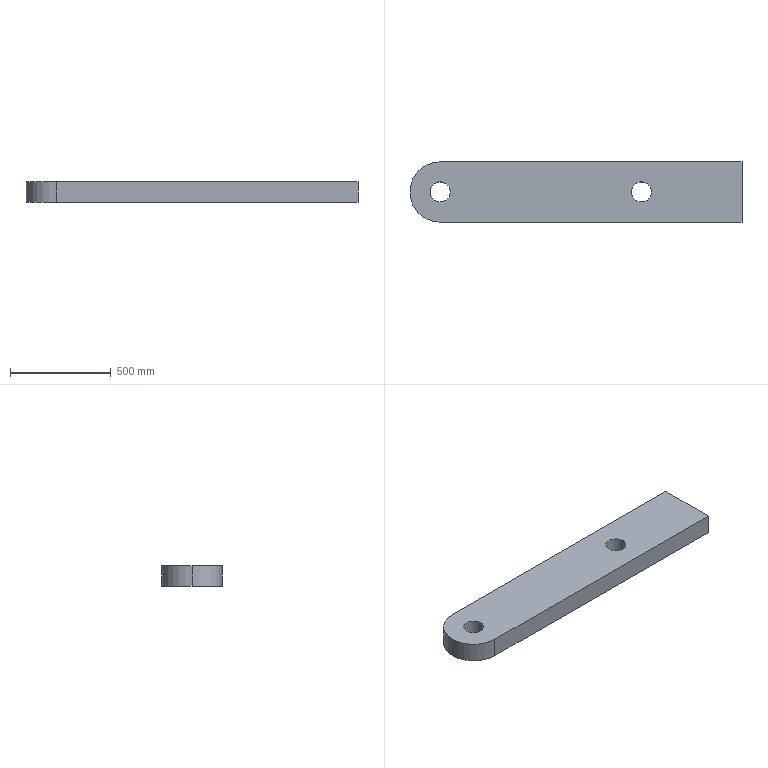Part | SolidWorks | features Extrusion 1 | 1 solid | 11 faces | box 1650 x 300 x 100 mm | volume 46963495 mm3 | cylinder 6 | plane 5 | commonest cylinder face diameters 100 x4 300 x2
STEP:
#1=CARTESIAN_POINT('',(-50.,0.,100.));
#2=VERTEX_POINT('',#1);
#3=CARTESIAN_POINT('',(50.,0.,100.));
#4=VERTEX_POINT('',#3);
#5=CARTESIAN_POINT('',(0.,0.,100.));
#6=DIRECTION('',(0.,0.,1.));
#7=DIRECTION('',(1.,0.,0.));
#8=AXIS2_PLACEMENT_3D('',#5,#6,#7);
#9=CIRCLE('',#8,50.);
#10=EDGE_CURVE('',#2,#4,#9,.T.);
#11=ORIENTED_EDGE('',*,*,#10,.T.);
#12=CARTESIAN_POINT('',(50.,0.,0.));
#13=VERTEX_POINT('',#12);
#14=CARTESIAN_POINT('',(50.,0.,100.));
#15=DIRECTION('',(0.,0.,-1.));
#16=VECTOR('',#15,1000.);
#17=LINE('',#14,#16);
#18=EDGE_CURVE('',#4,#13,#17,.T.);
#19=ORIENTED_EDGE('',*,*,#18,.T.);
#20=CARTESIAN_POINT('',(-50.,0.,0.));
#21=VERTEX_POINT('',#20);
#22=CARTESIAN_POINT('',(0.,0.,0.));
#23=DIRECTION('',(0.,0.,1.));
#24=DIRECTION('',(1.,0.,0.));
#25=AXIS2_PLACEMENT_3D('',#22,#23,#24);
#26=CIRCLE('',#25,50.);
#27=EDGE_CURVE('',#21,#13,#26,.T.);
#28=ORIENTED_EDGE('',*,*,#27,.F.);
#29=CARTESIAN_POINT('',(-50.,0.,100.));
#30=DIRECTION('',(0.,0.,-1.));
#31=VECTOR('',#30,1000.);
#32=LINE('',#29,#31);
#33=EDGE_CURVE('',#2,#21,#32,.T.);
#34=ORIENTED_EDGE('',*,*,#33,.F.);
#35=EDGE_LOOP('',(#11,#19,#28,#34));
#36=FACE_OUTER_BOUND('',#35,.T.);
#37=CARTESIAN_POINT('',(0.,0.,100.));
#38=DIRECTION('',(0.,0.,-1.));
#39=DIRECTION('',(-1.,0.,0.));
#40=AXIS2_PLACEMENT_3D('',#37,#38,#39);
#41=CYLINDRICAL_SURFACE('',#40,50.);
#42=ADVANCED_FACE('',(#36),#41,.F.);
#43=CARTESIAN_POINT('',(950.,0.,100.));
#44=VERTEX_POINT('',#43);
#45=CARTESIAN_POINT('',(1050.,0.,100.));
#46=VERTEX_POINT('',#45);
#47=CARTESIAN_POINT('',(1000.,0.,100.));
#48=DIRECTION('',(0.,0.,1.));
#49=DIRECTION('',(1.,0.,0.));
#50=AXIS2_PLACEMENT_3D('',#47,#48,#49);
#51=CIRCLE('',#50,50.);
#52=EDGE_CURVE('',#44,#46,#51,.T.);
#53=ORIENTED_EDGE('',*,*,#52,.T.);
#54=CARTESIAN_POINT('',(1050.,0.,0.));
#55=VERTEX_POINT('',#54);
#56=CARTESIAN_POINT('',(1050.,0.,100.));
#57=DIRECTION('',(0.,0.,-1.));
#58=VECTOR('',#57,1000.);
#59=LINE('',#56,#58);
#60=EDGE_CURVE('',#46,#55,#59,.T.);
#61=ORIENTED_EDGE('',*,*,#60,.T.);
#62=CARTESIAN_POINT('',(950.,0.,0.));
#63=VERTEX_POINT('',#62);
#64=CARTESIAN_POINT('',(1000.,0.,0.));
#65=DIRECTION('',(0.,0.,1.));
#66=DIRECTION('',(1.,0.,0.));
#67=AXIS2_PLACEMENT_3D('',#64,#65,#66);
#68=CIRCLE('',#67,50.);
#69=EDGE_CURVE('',#63,#55,#68,.T.);
#70=ORIENTED_EDGE('',*,*,#69,.F.);
#71=CARTESIAN_POINT('',(950.,0.,100.));
#72=DIRECTION('',(0.,0.,-1.));
#73=VECTOR('',#72,1000.);
#74=LINE('',#71,#73);
#75=EDGE_CURVE('',#44,#63,#74,.T.);
#76=ORIENTED_EDGE('',*,*,#75,.F.);
#77=EDGE_LOOP('',(#53,#61,#70,#76));
#78=FACE_OUTER_BOUND('',#77,.T.);
#79=CARTESIAN_POINT('',(1000.,0.,100.));
#80=DIRECTION('',(0.,0.,-1.));
#81=DIRECTION('',(-1.,0.,0.));
#82=AXIS2_PLACEMENT_3D('',#79,#80,#81);
#83=CYLINDRICAL_SURFACE('',#82,50.);
#84=ADVANCED_FACE('',(#78),#83,.F.);
#85=CARTESIAN_POINT('',(-150.,0.,100.));
#86=VERTEX_POINT('',#85);
#87=CARTESIAN_POINT('',(0.,-150.,100.));
#88=VERTEX_POINT('',#87);
#89=CARTESIAN_POINT('',(0.,0.,100.));
#90=DIRECTION('',(0.,0.,1.));
#91=DIRECTION('',(1.,0.,0.));
#92=AXIS2_PLACEMENT_3D('',#89,#90,#91);
#93=CIRCLE('',#92,150.);
#94=EDGE_CURVE('',#86,#88,#93,.T.);
#95=ORIENTED_EDGE('',*,*,#94,.F.);
#96=CARTESIAN_POINT('',(-150.,0.,0.));
#97=VERTEX_POINT('',#96);
#98=CARTESIAN_POINT('',(-150.,0.,100.));
#99=DIRECTION('',(0.,0.,-1.));
#100=VECTOR('',#99,1000.);
#101=LINE('',#98,#100);
#102=EDGE_CURVE('',#86,#97,#101,.T.);
#103=ORIENTED_EDGE('',*,*,#102,.T.);
#104=CARTESIAN_POINT('',(0.,-150.,0.));
#105=VERTEX_POINT('',#104);
#106=CARTESIAN_POINT('',(0.,0.,0.));
#107=DIRECTION('',(0.,0.,1.));
#108=DIRECTION('',(1.,0.,0.));
#109=AXIS2_PLACEMENT_3D('',#106,#107,#108);
#110=CIRCLE('',#109,150.);
#111=EDGE_CURVE('',#97,#105,#110,.T.);
#112=ORIENTED_EDGE('',*,*,#111,.T.);
#113=CARTESIAN_POINT('',(0.,-150.,100.));
#114=DIRECTION('',(0.,0.,-1.));
#115=VECTOR('',#114,1000.);
#116=LINE('',#113,#115);
#117=EDGE_CURVE('',#88,#105,#116,.T.);
#118=ORIENTED_EDGE('',*,*,#117,.F.);
#119=EDGE_LOOP('',(#95,#103,#112,#118));
#120=FACE_OUTER_BOUND('',#119,.T.);
#121=CARTESIAN_POINT('',(0.,0.,100.));
#122=DIRECTION('',(0.,0.,-1.));
#123=DIRECTION('',(-1.,0.,0.));
#124=AXIS2_PLACEMENT_3D('',#121,#122,#123);
#125=CYLINDRICAL_SURFACE('',#124,150.);
#126=ADVANCED_FACE('',(#120),#125,.T.);
#127=ORIENTED_EDGE('',*,*,#52,.F.);
#128=CARTESIAN_POINT('',(1000.,0.,100.));
#129=DIRECTION('',(0.,0.,1.));
#130=DIRECTION('',(1.,0.,0.));
#131=AXIS2_PLACEMENT_3D('',#128,#129,#130);
#132=CIRCLE('',#131,50.);
#133=EDGE_CURVE('',#46,#44,#132,.T.);
#134=ORIENTED_EDGE('',*,*,#133,.F.);
#135=EDGE_LOOP('',(#127,#134));
#136=FACE_BOUND('',#135,.T.);
#137=CARTESIAN_POINT('',(0.,150.,100.));
#138=VERTEX_POINT('',#137);
#139=CARTESIAN_POINT('',(0.,0.,100.));
#140=DIRECTION('',(0.,0.,1.));
#141=DIRECTION('',(1.,0.,0.));
#142=AXIS2_PLACEMENT_3D('',#139,#140,#141);
#143=CIRCLE('',#142,150.);
#144=EDGE_CURVE('',#138,#86,#143,.T.);
#145=ORIENTED_EDGE('',*,*,#144,.T.);
#146=ORIENTED_EDGE('',*,*,#94,.T.);
#147=CARTESIAN_POINT('',(1500.,-150.,100.));
#148=VERTEX_POINT('',#147);
#149=CARTESIAN_POINT('',(1500.,-150.,100.));
#150=DIRECTION('',(1.,0.,0.));
#151=VECTOR('',#150,1000.);
#152=LINE('',#149,#151);
#153=EDGE_CURVE('',#88,#148,#152,.T.);
#154=ORIENTED_EDGE('',*,*,#153,.T.);
#155=CARTESIAN_POINT('',(1500.,150.,100.));
#156=VERTEX_POINT('',#155);
#157=CARTESIAN_POINT('',(1500.,150.,100.));
#158=DIRECTION('',(0.,1.,0.));
#159=VECTOR('',#158,1000.);
#160=LINE('',#157,#159);
#161=EDGE_CURVE('',#148,#156,#160,.T.);
#162=ORIENTED_EDGE('',*,*,#161,.T.);
#163=CARTESIAN_POINT('',(0.,150.,100.));
#164=DIRECTION('',(-1.,0.,0.));
#165=VECTOR('',#164,1000.);
#166=LINE('',#163,#165);
#167=EDGE_CURVE('',#156,#138,#166,.T.);
#168=ORIENTED_EDGE('',*,*,#167,.T.);
#169=EDGE_LOOP('',(#145,#146,#154,#162,#168));
#170=FACE_OUTER_BOUND('',#169,.T.);
#171=ORIENTED_EDGE('',*,*,#10,.F.);
#172=CARTESIAN_POINT('',(0.,0.,100.));
#173=DIRECTION('',(0.,0.,1.));
#174=DIRECTION('',(1.,0.,0.));
#175=AXIS2_PLACEMENT_3D('',#172,#173,#174);
#176=CIRCLE('',#175,50.);
#177=EDGE_CURVE('',#4,#2,#176,.T.);
#178=ORIENTED_EDGE('',*,*,#177,.F.);
#179=EDGE_LOOP('',(#171,#178));
#180=FACE_BOUND('',#179,.T.);
#181=CARTESIAN_POINT('',(0.,0.,100.));
#182=DIRECTION('',(0.,0.,1.));
#183=DIRECTION('',(1.,0.,0.));
#184=AXIS2_PLACEMENT_3D('',#181,#182,#183);
#185=PLANE('',#184);
#186=ADVANCED_FACE('',(#136,#170,#180),#185,.T.);
#187=ORIENTED_EDGE('',*,*,#69,.T.);
#188=CARTESIAN_POINT('',(1000.,0.,0.));
#189=DIRECTION('',(0.,0.,1.));
#190=DIRECTION('',(1.,0.,0.));
#191=AXIS2_PLACEMENT_3D('',#188,#189,#190);
#192=CIRCLE('',#191,50.);
#193=EDGE_CURVE('',#55,#63,#192,.T.);
#194=ORIENTED_EDGE('',*,*,#193,.T.);
#195=EDGE_LOOP('',(#187,#194));
#196=FACE_BOUND('',#195,.T.);
#197=CARTESIAN_POINT('',(0.,150.,0.));
#198=VERTEX_POINT('',#197);
#199=CARTESIAN_POINT('',(0.,0.,0.));
#200=DIRECTION('',(0.,0.,1.));
#201=DIRECTION('',(1.,0.,0.));
#202=AXIS2_PLACEMENT_3D('',#199,#200,#201);
#203=CIRCLE('',#202,150.);
#204=EDGE_CURVE('',#198,#97,#203,.T.);
#205=ORIENTED_EDGE('',*,*,#204,.F.);
#206=CARTESIAN_POINT('',(1500.,150.,0.));
#207=VERTEX_POINT('',#206);
#208=CARTESIAN_POINT('',(0.,150.,0.));
#209=DIRECTION('',(-1.,0.,0.));
#210=VECTOR('',#209,1000.);
#211=LINE('',#208,#210);
#212=EDGE_CURVE('',#207,#198,#211,.T.);
#213=ORIENTED_EDGE('',*,*,#212,.F.);
#214=CARTESIAN_POINT('',(1500.,-150.,0.));
#215=VERTEX_POINT('',#214);
#216=CARTESIAN_POINT('',(1500.,150.,0.));
#217=DIRECTION('',(0.,1.,0.));
#218=VECTOR('',#217,1000.);
#219=LINE('',#216,#218);
#220=EDGE_CURVE('',#215,#207,#219,.T.);
#221=ORIENTED_EDGE('',*,*,#220,.F.);
#222=CARTESIAN_POINT('',(1500.,-150.,0.));
#223=DIRECTION('',(1.,0.,0.));
#224=VECTOR('',#223,1000.);
#225=LINE('',#222,#224);
#226=EDGE_CURVE('',#105,#215,#225,.T.);
#227=ORIENTED_EDGE('',*,*,#226,.F.);
#228=ORIENTED_EDGE('',*,*,#111,.F.);
#229=EDGE_LOOP('',(#205,#213,#221,#227,#228));
#230=FACE_OUTER_BOUND('',#229,.T.);
#231=ORIENTED_EDGE('',*,*,#27,.T.);
#232=CARTESIAN_POINT('',(0.,0.,0.));
#233=DIRECTION('',(0.,0.,1.));
#234=DIRECTION('',(1.,0.,0.));
#235=AXIS2_PLACEMENT_3D('',#232,#233,#234);
#236=CIRCLE('',#235,50.);
#237=EDGE_CURVE('',#13,#21,#236,.T.);
#238=ORIENTED_EDGE('',*,*,#237,.T.);
#239=EDGE_LOOP('',(#231,#238));
#240=FACE_BOUND('',#239,.T.);
#241=CARTESIAN_POINT('',(0.,0.,0.));
#242=DIRECTION('',(0.,0.,1.));
#243=DIRECTION('',(1.,0.,0.));
#244=AXIS2_PLACEMENT_3D('',#241,#242,#243);
#245=PLANE('',#244);
#246=ADVANCED_FACE('',(#196,#230,#240),#245,.F.);
#247=ORIENTED_EDGE('',*,*,#102,.F.);
#248=ORIENTED_EDGE('',*,*,#144,.F.);
#249=CARTESIAN_POINT('',(0.,150.,100.));
#250=DIRECTION('',(0.,0.,-1.));
#251=VECTOR('',#250,1000.);
#252=LINE('',#249,#251);
#253=EDGE_CURVE('',#138,#198,#252,.T.);
#254=ORIENTED_EDGE('',*,*,#253,.T.);
#255=ORIENTED_EDGE('',*,*,#204,.T.);
#256=EDGE_LOOP('',(#247,#248,#254,#255));
#257=FACE_OUTER_BOUND('',#256,.T.);
#258=CARTESIAN_POINT('',(0.,0.,100.));
#259=DIRECTION('',(0.,0.,-1.));
#260=DIRECTION('',(-1.,0.,0.));
#261=AXIS2_PLACEMENT_3D('',#258,#259,#260);
#262=CYLINDRICAL_SURFACE('',#261,150.);
#263=ADVANCED_FACE('',(#257),#262,.T.);
#264=ORIENTED_EDGE('',*,*,#226,.T.);
#265=CARTESIAN_POINT('',(1500.,-150.,100.));
#266=DIRECTION('',(0.,0.,-1.));
#267=VECTOR('',#266,1000.);
#268=LINE('',#265,#267);
#269=EDGE_CURVE('',#148,#215,#268,.T.);
#270=ORIENTED_EDGE('',*,*,#269,.F.);
#271=ORIENTED_EDGE('',*,*,#153,.F.);
#272=ORIENTED_EDGE('',*,*,#117,.T.);
#273=EDGE_LOOP('',(#264,#270,#271,#272));
#274=FACE_OUTER_BOUND('',#273,.T.);
#275=CARTESIAN_POINT('',(1500.,-150.,100.));
#276=DIRECTION('',(0.,1.,0.));
#277=DIRECTION('',(-1.,0.,0.));
#278=AXIS2_PLACEMENT_3D('',#275,#276,#277);
#279=PLANE('',#278);
#280=ADVANCED_FACE('',(#274),#279,.F.);
#281=ORIENTED_EDGE('',*,*,#220,.T.);
#282=CARTESIAN_POINT('',(1500.,150.,100.));
#283=DIRECTION('',(0.,0.,-1.));
#284=VECTOR('',#283,1000.);
#285=LINE('',#282,#284);
#286=EDGE_CURVE('',#156,#207,#285,.T.);
#287=ORIENTED_EDGE('',*,*,#286,.F.);
#288=ORIENTED_EDGE('',*,*,#161,.F.);
#289=ORIENTED_EDGE('',*,*,#269,.T.);
#290=EDGE_LOOP('',(#281,#287,#288,#289));
#291=FACE_OUTER_BOUND('',#290,.T.);
#292=CARTESIAN_POINT('',(1500.,150.,100.));
#293=DIRECTION('',(-1.,0.,0.));
#294=DIRECTION('',(0.,0.,1.));
#295=AXIS2_PLACEMENT_3D('',#292,#293,#294);
#296=PLANE('',#295);
#297=ADVANCED_FACE('',(#291),#296,.F.);
#298=ORIENTED_EDGE('',*,*,#212,.T.);
#299=ORIENTED_EDGE('',*,*,#253,.F.);
#300=ORIENTED_EDGE('',*,*,#167,.F.);
#301=ORIENTED_EDGE('',*,*,#286,.T.);
#302=EDGE_LOOP('',(#298,#299,#300,#301));
#303=FACE_OUTER_BOUND('',#302,.T.);
#304=CARTESIAN_POINT('',(0.,150.,100.));
#305=DIRECTION('',(0.,-1.,0.));
#306=DIRECTION('',(1.,0.,0.));
#307=AXIS2_PLACEMENT_3D('',#304,#305,#306);
#308=PLANE('',#307);
#309=ADVANCED_FACE('',(#303),#308,.F.);
#310=ORIENTED_EDGE('',*,*,#60,.F.);
#311=ORIENTED_EDGE('',*,*,#133,.T.);
#312=ORIENTED_EDGE('',*,*,#75,.T.);
#313=ORIENTED_EDGE('',*,*,#193,.F.);
#314=EDGE_LOOP('',(#310,#311,#312,#313));
#315=FACE_OUTER_BOUND('',#314,.T.);
#316=CARTESIAN_POINT('',(1000.,0.,100.));
#317=DIRECTION('',(0.,0.,-1.));
#318=DIRECTION('',(-1.,0.,0.));
#319=AXIS2_PLACEMENT_3D('',#316,#317,#318);
#320=CYLINDRICAL_SURFACE('',#319,50.);
#321=ADVANCED_FACE('',(#315),#320,.F.);
#322=ORIENTED_EDGE('',*,*,#18,.F.);
#323=ORIENTED_EDGE('',*,*,#177,.T.);
#324=ORIENTED_EDGE('',*,*,#33,.T.);
#325=ORIENTED_EDGE('',*,*,#237,.F.);
#326=EDGE_LOOP('',(#322,#323,#324,#325));
#327=FACE_OUTER_BOUND('',#326,.T.);
#328=CARTESIAN_POINT('',(0.,0.,100.));
#329=DIRECTION('',(0.,0.,-1.));
#330=DIRECTION('',(-1.,0.,0.));
#331=AXIS2_PLACEMENT_3D('',#328,#329,#330);
#332=CYLINDRICAL_SURFACE('',#331,50.);
#333=ADVANCED_FACE('',(#327),#332,.F.);
#334=CLOSED_SHELL('',(#42,#84,#126,#186,#246,#263,#280,#297,#309,#321,#333));
#335=MANIFOLD_SOLID_BREP('',#334);
#336=CARTESIAN_POINT('',(0.,0.,0.));
#337=DIRECTION('',(0.,0.,1.));
#338=DIRECTION('',(1.,0.,0.));
#339=AXIS2_PLACEMENT_3D('',#336,#337,#338);
#340=(LENGTH_UNIT()NAMED_UNIT(*)SI_UNIT(.MILLI.,.METRE.));
#341=UNCERTAINTY_MEASURE_WITH_UNIT(LENGTH_MEASURE(0.00001),#340,'','');
#342=(NAMED_UNIT(*)PLANE_ANGLE_UNIT()SI_UNIT($,.RADIAN.));
#343=(NAMED_UNIT(*)SI_UNIT($,.STERADIAN.)SOLID_ANGLE_UNIT());
#344=(GEOMETRIC_REPRESENTATION_CONTEXT(3)GLOBAL_UNCERTAINTY_ASSIGNED_CONTEXT((#341))GLOBAL_UNIT_ASSIGNED_CONTEXT((#340,#342,#343))REPRESENTATION_CONTEXT('',''));
#345=ADVANCED_BREP_SHAPE_REPRESENTATION('',(#335,#339),#344);